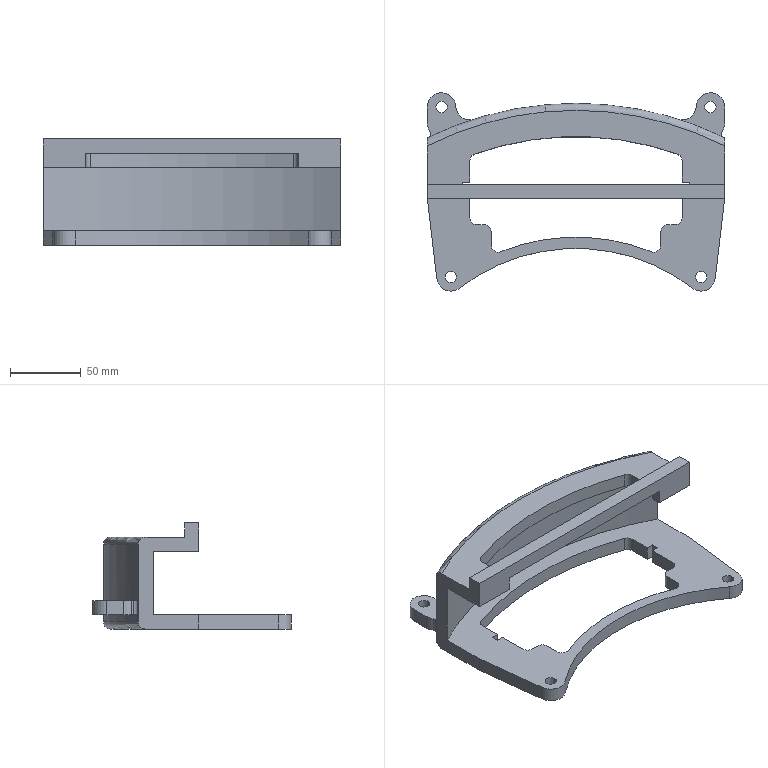Part | SolidWorks | features ICE 5, Fillet 4, Cut 1, Extrusion 1, Shell 1 | 1 solid | 80 faces | box 210 x 140.109 x 75 mm | volume 309603 mm3 | plane 42 | cylinder 36 | torus 2 | commonest cylinder face diameters 10 x10 8 x8 20 x8 6 x4 428 x2 270 x1